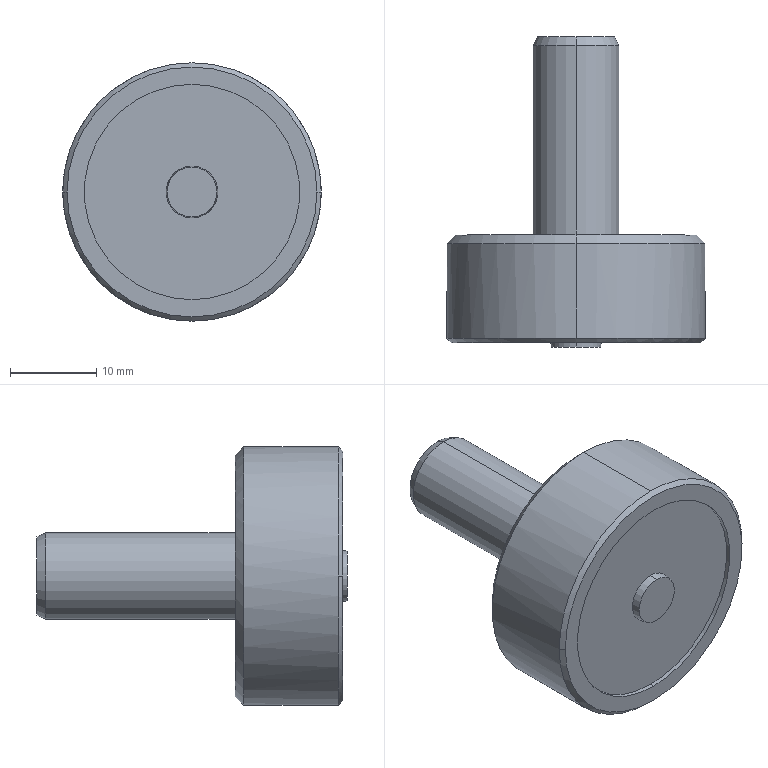Part | SolidWorks | features BaseBody 1 | 1 solid | 19 faces | box 30 x 36 x 30 mm | volume 10359 mm3 | cone 8 | cylinder 6 | plane 5 | commonest cylinder face diameters 10 x2 25 x2 30 x2
STEP:
#1=CARTESIAN_POINT('',(-257.5,37.,118.121));
#2=VERTEX_POINT('',#1);
#3=CARTESIAN_POINT('',(-257.5,37.,128.121));
#4=VERTEX_POINT('',#3);
#5=CARTESIAN_POINT('',(-257.5,37.,123.121));
#6=DIRECTION('',(0.,-1.,0.));
#7=DIRECTION('',(0.,0.,1.));
#8=AXIS2_PLACEMENT_3D('',#5,#6,#7);
#9=CIRCLE('',#8,5.);
#10=EDGE_CURVE('',#2,#4,#9,.T.);
#11=ORIENTED_EDGE('',*,*,#10,.F.);
#12=CARTESIAN_POINT('',(-257.5,59.,118.121));
#13=VERTEX_POINT('',#12);
#14=CARTESIAN_POINT('',(-257.5,60.,118.121));
#15=DIRECTION('',(0.,1.,0.));
#16=VECTOR('',#15,1000.);
#17=LINE('',#14,#16);
#18=EDGE_CURVE('',#2,#13,#17,.T.);
#19=ORIENTED_EDGE('',*,*,#18,.T.);
#20=CARTESIAN_POINT('',(-257.5,59.,128.121));
#21=VERTEX_POINT('',#20);
#22=CARTESIAN_POINT('',(-257.5,59.,123.121));
#23=DIRECTION('',(0.,-1.,0.));
#24=DIRECTION('',(0.,0.,1.));
#25=AXIS2_PLACEMENT_3D('',#22,#23,#24);
#26=CIRCLE('',#25,5.);
#27=EDGE_CURVE('',#13,#21,#26,.T.);
#28=ORIENTED_EDGE('',*,*,#27,.T.);
#29=CARTESIAN_POINT('',(-257.5,60.,128.121));
#30=DIRECTION('',(0.,1.,0.));
#31=VECTOR('',#30,1000.);
#32=LINE('',#29,#31);
#33=EDGE_CURVE('',#4,#21,#32,.T.);
#34=ORIENTED_EDGE('',*,*,#33,.F.);
#35=EDGE_LOOP('',(#11,#19,#28,#34));
#36=FACE_OUTER_BOUND('',#35,.T.);
#37=CARTESIAN_POINT('',(-257.5,60.,123.121));
#38=DIRECTION('',(0.,1.,0.));
#39=DIRECTION('',(0.,0.,1.));
#40=AXIS2_PLACEMENT_3D('',#37,#38,#39);
#41=CYLINDRICAL_SURFACE('',#40,5.);
#42=ADVANCED_FACE('',(#36),#41,.T.);
#43=CARTESIAN_POINT('',(-257.5,37.,137.121));
#44=VERTEX_POINT('',#43);
#45=CARTESIAN_POINT('',(-257.5,37.,109.121));
#46=VERTEX_POINT('',#45);
#47=CARTESIAN_POINT('',(-257.5,37.,123.121));
#48=DIRECTION('',(0.,1.,0.));
#49=DIRECTION('',(0.,0.,-1.));
#50=AXIS2_PLACEMENT_3D('',#47,#48,#49);
#51=CIRCLE('',#50,14.);
#52=EDGE_CURVE('',#44,#46,#51,.T.);
#53=ORIENTED_EDGE('',*,*,#52,.F.);
#54=CARTESIAN_POINT('',(-257.5,36.,138.121));
#55=VERTEX_POINT('',#54);
#56=CARTESIAN_POINT('',(-257.5,36.,138.121));
#57=DIRECTION('',(0.,-0.7071,0.7071));
#58=VECTOR('',#57,1000.);
#59=LINE('',#56,#58);
#60=EDGE_CURVE('',#44,#55,#59,.T.);
#61=ORIENTED_EDGE('',*,*,#60,.T.);
#62=CARTESIAN_POINT('',(-257.5,36.,108.121));
#63=VERTEX_POINT('',#62);
#64=CARTESIAN_POINT('',(-257.5,36.,123.121));
#65=DIRECTION('',(0.,1.,0.));
#66=DIRECTION('',(-0.05078,0.,-0.9987));
#67=AXIS2_PLACEMENT_3D('',#64,#65,#66);
#68=CIRCLE('',#67,15.);
#69=EDGE_CURVE('',#55,#63,#68,.T.);
#70=ORIENTED_EDGE('',*,*,#69,.T.);
#71=CARTESIAN_POINT('',(-257.5,36.,108.121));
#72=DIRECTION('',(0.,-0.7071,-0.7071));
#73=VECTOR('',#72,1000.);
#74=LINE('',#71,#73);
#75=EDGE_CURVE('',#46,#63,#74,.T.);
#76=ORIENTED_EDGE('',*,*,#75,.F.);
#77=EDGE_LOOP('',(#53,#61,#70,#76));
#78=FACE_OUTER_BOUND('',#77,.T.);
#79=CARTESIAN_POINT('',(-257.5,36.,123.121));
#80=DIRECTION('',(0.,-1.,0.));
#81=DIRECTION('',(0.,0.,-1.));
#82=AXIS2_PLACEMENT_3D('',#79,#80,#81);
#83=CONICAL_SURFACE('',#82,15.,0.7854);
#84=ADVANCED_FACE('',(#78),#83,.T.);
#85=CARTESIAN_POINT('',(-257.5,60.,118.587));
#86=VERTEX_POINT('',#85);
#87=CARTESIAN_POINT('',(-257.5,60.,127.655));
#88=VERTEX_POINT('',#87);
#89=CARTESIAN_POINT('',(-257.5,60.,123.121));
#90=DIRECTION('',(0.,-1.,0.));
#91=DIRECTION('',(0.,0.,-1.));
#92=AXIS2_PLACEMENT_3D('',#89,#90,#91);
#93=CIRCLE('',#92,4.534);
#94=EDGE_CURVE('',#86,#88,#93,.T.);
#95=ORIENTED_EDGE('',*,*,#94,.T.);
#96=CARTESIAN_POINT('',(-257.5,59.,128.121));
#97=DIRECTION('',(0.,-0.9063,0.4226));
#98=VECTOR('',#97,1000.);
#99=LINE('',#96,#98);
#100=EDGE_CURVE('',#88,#21,#99,.T.);
#101=ORIENTED_EDGE('',*,*,#100,.T.);
#102=ORIENTED_EDGE('',*,*,#27,.F.);
#103=CARTESIAN_POINT('',(-257.5,59.,118.121));
#104=DIRECTION('',(0.,-0.9063,-0.4226));
#105=VECTOR('',#104,1000.);
#106=LINE('',#103,#105);
#107=EDGE_CURVE('',#86,#13,#106,.T.);
#108=ORIENTED_EDGE('',*,*,#107,.F.);
#109=EDGE_LOOP('',(#95,#101,#102,#108));
#110=FACE_OUTER_BOUND('',#109,.T.);
#111=CARTESIAN_POINT('',(-257.5,59.,123.121));
#112=DIRECTION('',(0.,-1.,0.));
#113=DIRECTION('',(0.,0.,-1.));
#114=AXIS2_PLACEMENT_3D('',#111,#112,#113);
#115=CONICAL_SURFACE('',#114,5.,0.4363);
#116=ADVANCED_FACE('',(#110),#115,.T.);
#117=CARTESIAN_POINT('',(-242.5,25.,123.121));
#118=VERTEX_POINT('',#117);
#119=CARTESIAN_POINT('',(-257.5,25.,108.121));
#120=VERTEX_POINT('',#119);
#121=CARTESIAN_POINT('',(-257.5,25.,123.121));
#122=DIRECTION('',(0.,1.,0.));
#123=DIRECTION('',(0.,0.,1.));
#124=AXIS2_PLACEMENT_3D('',#121,#122,#123);
#125=CIRCLE('',#124,15.);
#126=EDGE_CURVE('',#118,#120,#125,.T.);
#127=ORIENTED_EDGE('',*,*,#126,.T.);
#128=CARTESIAN_POINT('',(-257.5,60.,108.121));
#129=DIRECTION('',(0.,1.,0.));
#130=VECTOR('',#129,1000.);
#131=LINE('',#128,#130);
#132=EDGE_CURVE('',#120,#63,#131,.T.);
#133=ORIENTED_EDGE('',*,*,#132,.T.);
#134=ORIENTED_EDGE('',*,*,#69,.F.);
#135=CARTESIAN_POINT('',(-257.5,25.,138.121));
#136=VERTEX_POINT('',#135);
#137=CARTESIAN_POINT('',(-257.5,60.,138.121));
#138=DIRECTION('',(0.,1.,0.));
#139=VECTOR('',#138,1000.);
#140=LINE('',#137,#139);
#141=EDGE_CURVE('',#136,#55,#140,.T.);
#142=ORIENTED_EDGE('',*,*,#141,.F.);
#143=CARTESIAN_POINT('',(-257.5,25.,123.121));
#144=DIRECTION('',(0.,1.,0.));
#145=DIRECTION('',(0.,0.,1.));
#146=AXIS2_PLACEMENT_3D('',#143,#144,#145);
#147=CIRCLE('',#146,15.);
#148=EDGE_CURVE('',#136,#118,#147,.T.);
#149=ORIENTED_EDGE('',*,*,#148,.T.);
#150=EDGE_LOOP('',(#127,#133,#134,#142,#149));
#151=FACE_OUTER_BOUND('',#150,.T.);
#152=CARTESIAN_POINT('',(-257.5,60.,123.121));
#153=DIRECTION('',(0.,1.,0.));
#154=DIRECTION('',(0.,0.,1.));
#155=AXIS2_PLACEMENT_3D('',#152,#153,#154);
#156=CYLINDRICAL_SURFACE('',#155,15.);
#157=ADVANCED_FACE('',(#151),#156,.T.);
#158=CARTESIAN_POINT('',(-272.,24.5,123.121));
#159=VERTEX_POINT('',#158);
#160=CARTESIAN_POINT('',(-243.,24.5,123.121));
#161=VERTEX_POINT('',#160);
#162=CARTESIAN_POINT('',(-257.5,24.5,123.121));
#163=DIRECTION('',(0.,1.,0.));
#164=DIRECTION('',(-1.,0.,0.));
#165=AXIS2_PLACEMENT_3D('',#162,#163,#164);
#166=CIRCLE('',#165,14.5);
#167=EDGE_CURVE('',#159,#161,#166,.T.);
#168=ORIENTED_EDGE('',*,*,#167,.T.);
#169=CARTESIAN_POINT('',(-242.5,25.,123.121));
#170=DIRECTION('',(0.7071,0.7071,0.));
#171=VECTOR('',#170,1000.);
#172=LINE('',#169,#171);
#173=EDGE_CURVE('',#161,#118,#172,.T.);
#174=ORIENTED_EDGE('',*,*,#173,.T.);
#175=ORIENTED_EDGE('',*,*,#148,.F.);
#176=CARTESIAN_POINT('',(-272.5,25.,123.121));
#177=VERTEX_POINT('',#176);
#178=CARTESIAN_POINT('',(-257.5,25.,123.121));
#179=DIRECTION('',(0.,1.,0.));
#180=DIRECTION('',(0.,0.,1.));
#181=AXIS2_PLACEMENT_3D('',#178,#179,#180);
#182=CIRCLE('',#181,15.);
#183=EDGE_CURVE('',#177,#136,#182,.T.);
#184=ORIENTED_EDGE('',*,*,#183,.F.);
#185=CARTESIAN_POINT('',(-272.5,25.,123.121));
#186=DIRECTION('',(-0.7071,0.7071,0.));
#187=VECTOR('',#186,1000.);
#188=LINE('',#185,#187);
#189=EDGE_CURVE('',#159,#177,#188,.T.);
#190=ORIENTED_EDGE('',*,*,#189,.F.);
#191=EDGE_LOOP('',(#168,#174,#175,#184,#190));
#192=FACE_OUTER_BOUND('',#191,.T.);
#193=CARTESIAN_POINT('',(-257.5,25.,123.121));
#194=DIRECTION('',(0.,1.,0.));
#195=DIRECTION('',(-1.,0.,0.));
#196=AXIS2_PLACEMENT_3D('',#193,#194,#195);
#197=CONICAL_SURFACE('',#196,15.,0.7854);
#198=ADVANCED_FACE('',(#192),#197,.T.);
#199=CARTESIAN_POINT('',(-257.5,25.,135.621));
#200=VERTEX_POINT('',#199);
#201=CARTESIAN_POINT('',(-257.5,25.,110.621));
#202=VERTEX_POINT('',#201);
#203=CARTESIAN_POINT('',(-257.5,25.,123.121));
#204=DIRECTION('',(0.,-1.,0.));
#205=DIRECTION('',(0.,0.,-1.));
#206=AXIS2_PLACEMENT_3D('',#203,#204,#205);
#207=CIRCLE('',#206,12.5);
#208=EDGE_CURVE('',#200,#202,#207,.T.);
#209=ORIENTED_EDGE('',*,*,#208,.F.);
#210=CARTESIAN_POINT('',(-257.5,24.5,135.621));
#211=VERTEX_POINT('',#210);
#212=CARTESIAN_POINT('',(-257.5,25.,135.621));
#213=DIRECTION('',(0.,-1.,0.));
#214=VECTOR('',#213,1000.);
#215=LINE('',#212,#214);
#216=EDGE_CURVE('',#200,#211,#215,.T.);
#217=ORIENTED_EDGE('',*,*,#216,.T.);
#218=CARTESIAN_POINT('',(-257.5,24.5,110.621));
#219=VERTEX_POINT('',#218);
#220=CARTESIAN_POINT('',(-257.5,24.5,123.121));
#221=DIRECTION('',(0.,1.,0.));
#222=DIRECTION('',(0.,0.,-1.));
#223=AXIS2_PLACEMENT_3D('',#220,#221,#222);
#224=CIRCLE('',#223,12.5);
#225=EDGE_CURVE('',#219,#211,#224,.T.);
#226=ORIENTED_EDGE('',*,*,#225,.F.);
#227=CARTESIAN_POINT('',(-257.5,25.,110.621));
#228=DIRECTION('',(0.,-1.,0.));
#229=VECTOR('',#228,1000.);
#230=LINE('',#227,#229);
#231=EDGE_CURVE('',#202,#219,#230,.T.);
#232=ORIENTED_EDGE('',*,*,#231,.F.);
#233=EDGE_LOOP('',(#209,#217,#226,#232));
#234=FACE_OUTER_BOUND('',#233,.T.);
#235=CARTESIAN_POINT('',(-257.5,25.,123.121));
#236=DIRECTION('',(0.,-1.,0.));
#237=DIRECTION('',(0.,0.,-1.));
#238=AXIS2_PLACEMENT_3D('',#235,#236,#237);
#239=CYLINDRICAL_SURFACE('',#238,12.5);
#240=ADVANCED_FACE('',(#234),#239,.F.);
#241=CARTESIAN_POINT('',(-257.5,24.,126.016));
#242=VERTEX_POINT('',#241);
#243=CARTESIAN_POINT('',(-257.5,24.,120.226));
#244=VERTEX_POINT('',#243);
#245=CARTESIAN_POINT('',(-257.5,24.,123.121));
#246=DIRECTION('',(0.,1.,0.));
#247=DIRECTION('',(0.,0.,1.));
#248=AXIS2_PLACEMENT_3D('',#245,#246,#247);
#249=CIRCLE('',#248,2.895);
#250=EDGE_CURVE('',#242,#244,#249,.T.);
#251=ORIENTED_EDGE('',*,*,#250,.T.);
#252=CARTESIAN_POINT('',(-257.5,25.,120.121));
#253=VERTEX_POINT('',#252);
#254=CARTESIAN_POINT('',(-257.5,25.,120.121));
#255=DIRECTION('',(0.,0.9945,-0.1045));
#256=VECTOR('',#255,1000.);
#257=LINE('',#254,#256);
#258=EDGE_CURVE('',#244,#253,#257,.T.);
#259=ORIENTED_EDGE('',*,*,#258,.T.);
#260=CARTESIAN_POINT('',(-257.5,25.,126.121));
#261=VERTEX_POINT('',#260);
#262=CARTESIAN_POINT('',(-257.5,25.,123.121));
#263=DIRECTION('',(0.,1.,0.));
#264=DIRECTION('',(0.,0.,1.));
#265=AXIS2_PLACEMENT_3D('',#262,#263,#264);
#266=CIRCLE('',#265,3.);
#267=EDGE_CURVE('',#261,#253,#266,.T.);
#268=ORIENTED_EDGE('',*,*,#267,.F.);
#269=CARTESIAN_POINT('',(-257.5,25.,126.121));
#270=DIRECTION('',(0.,0.9945,0.1045));
#271=VECTOR('',#270,1000.);
#272=LINE('',#269,#271);
#273=EDGE_CURVE('',#242,#261,#272,.T.);
#274=ORIENTED_EDGE('',*,*,#273,.F.);
#275=EDGE_LOOP('',(#251,#259,#268,#274));
#276=FACE_OUTER_BOUND('',#275,.T.);
#277=CARTESIAN_POINT('',(-257.5,25.,123.121));
#278=DIRECTION('',(0.,1.,0.));
#279=DIRECTION('',(0.,0.,1.));
#280=AXIS2_PLACEMENT_3D('',#277,#278,#279);
#281=CONICAL_SURFACE('',#280,3.,0.1047);
#282=ADVANCED_FACE('',(#276),#281,.T.);
#283=CARTESIAN_POINT('',(-257.5,37.,123.121));
#284=DIRECTION('',(0.,-1.,0.));
#285=DIRECTION('',(0.,0.,1.));
#286=AXIS2_PLACEMENT_3D('',#283,#284,#285);
#287=CIRCLE('',#286,5.);
#288=EDGE_CURVE('',#4,#2,#287,.T.);
#289=ORIENTED_EDGE('',*,*,#288,.T.);
#290=ORIENTED_EDGE('',*,*,#10,.T.);
#291=EDGE_LOOP('',(#289,#290));
#292=FACE_BOUND('',#291,.T.);
#293=CARTESIAN_POINT('',(-257.5,37.,123.121));
#294=DIRECTION('',(0.,1.,0.));
#295=DIRECTION('',(0.,0.,-1.));
#296=AXIS2_PLACEMENT_3D('',#293,#294,#295);
#297=CIRCLE('',#296,14.);
#298=EDGE_CURVE('',#46,#44,#297,.T.);
#299=ORIENTED_EDGE('',*,*,#298,.T.);
#300=ORIENTED_EDGE('',*,*,#52,.T.);
#301=EDGE_LOOP('',(#299,#300));
#302=FACE_OUTER_BOUND('',#301,.T.);
#303=CARTESIAN_POINT('',(-256.738,37.,138.102));
#304=DIRECTION('',(0.,1.,0.));
#305=DIRECTION('',(0.,0.,1.));
#306=AXIS2_PLACEMENT_3D('',#303,#304,#305);
#307=PLANE('',#306);
#308=ADVANCED_FACE('',(#292,#302),#307,.T.);
#309=ORIENTED_EDGE('',*,*,#18,.F.);
#310=ORIENTED_EDGE('',*,*,#288,.F.);
#311=ORIENTED_EDGE('',*,*,#33,.T.);
#312=CARTESIAN_POINT('',(-257.5,59.,123.121));
#313=DIRECTION('',(0.,-1.,0.));
#314=DIRECTION('',(0.,0.,1.));
#315=AXIS2_PLACEMENT_3D('',#312,#313,#314);
#316=CIRCLE('',#315,5.);
#317=EDGE_CURVE('',#21,#13,#316,.T.);
#318=ORIENTED_EDGE('',*,*,#317,.T.);
#319=EDGE_LOOP('',(#309,#310,#311,#318));
#320=FACE_OUTER_BOUND('',#319,.T.);
#321=CARTESIAN_POINT('',(-257.5,60.,123.121));
#322=DIRECTION('',(0.,1.,0.));
#323=DIRECTION('',(0.,0.,1.));
#324=AXIS2_PLACEMENT_3D('',#321,#322,#323);
#325=CYLINDRICAL_SURFACE('',#324,5.);
#326=ADVANCED_FACE('',(#320),#325,.T.);
#327=ORIENTED_EDGE('',*,*,#60,.F.);
#328=ORIENTED_EDGE('',*,*,#298,.F.);
#329=ORIENTED_EDGE('',*,*,#75,.T.);
#330=CARTESIAN_POINT('',(-257.5,36.,123.121));
#331=DIRECTION('',(0.,1.,0.));
#332=DIRECTION('',(-0.05078,0.,-0.9987));
#333=AXIS2_PLACEMENT_3D('',#330,#331,#332);
#334=CIRCLE('',#333,15.);
#335=EDGE_CURVE('',#63,#55,#334,.T.);
#336=ORIENTED_EDGE('',*,*,#335,.T.);
#337=EDGE_LOOP('',(#327,#328,#329,#336));
#338=FACE_OUTER_BOUND('',#337,.T.);
#339=CARTESIAN_POINT('',(-257.5,36.,123.121));
#340=DIRECTION('',(0.,-1.,0.));
#341=DIRECTION('',(0.,0.,-1.));
#342=AXIS2_PLACEMENT_3D('',#339,#340,#341);
#343=CONICAL_SURFACE('',#342,15.,0.7854);
#344=ADVANCED_FACE('',(#338),#343,.T.);
#345=ORIENTED_EDGE('',*,*,#100,.F.);
#346=CARTESIAN_POINT('',(-257.5,60.,123.121));
#347=DIRECTION('',(0.,-1.,0.));
#348=DIRECTION('',(0.,0.,-1.));
#349=AXIS2_PLACEMENT_3D('',#346,#347,#348);
#350=CIRCLE('',#349,4.534);
#351=EDGE_CURVE('',#88,#86,#350,.T.);
#352=ORIENTED_EDGE('',*,*,#351,.T.);
#353=ORIENTED_EDGE('',*,*,#107,.T.);
#354=ORIENTED_EDGE('',*,*,#317,.F.);
#355=EDGE_LOOP('',(#345,#352,#353,#354));
#356=FACE_OUTER_BOUND('',#355,.T.);
#357=CARTESIAN_POINT('',(-257.5,59.,123.121));
#358=DIRECTION('',(0.,-1.,0.));
#359=DIRECTION('',(0.,0.,-1.));
#360=AXIS2_PLACEMENT_3D('',#357,#358,#359);
#361=CONICAL_SURFACE('',#360,5.,0.4363);
#362=ADVANCED_FACE('',(#356),#361,.T.);
#363=ORIENTED_EDGE('',*,*,#132,.F.);
#364=CARTESIAN_POINT('',(-257.5,25.,123.121));
#365=DIRECTION('',(0.,1.,0.));
#366=DIRECTION('',(0.,0.,1.));
#367=AXIS2_PLACEMENT_3D('',#364,#365,#366);
#368=CIRCLE('',#367,15.);
#369=EDGE_CURVE('',#120,#177,#368,.T.);
#370=ORIENTED_EDGE('',*,*,#369,.T.);
#371=ORIENTED_EDGE('',*,*,#183,.T.);
#372=ORIENTED_EDGE('',*,*,#141,.T.);
#373=ORIENTED_EDGE('',*,*,#335,.F.);
#374=EDGE_LOOP('',(#363,#370,#371,#372,#373));
#375=FACE_OUTER_BOUND('',#374,.T.);
#376=CARTESIAN_POINT('',(-257.5,60.,123.121));
#377=DIRECTION('',(0.,1.,0.));
#378=DIRECTION('',(0.,0.,1.));
#379=AXIS2_PLACEMENT_3D('',#376,#377,#378);
#380=CYLINDRICAL_SURFACE('',#379,15.);
#381=ADVANCED_FACE('',(#375),#380,.T.);
#382=ORIENTED_EDGE('',*,*,#94,.F.);
#383=ORIENTED_EDGE('',*,*,#351,.F.);
#384=EDGE_LOOP('',(#382,#383));
#385=FACE_OUTER_BOUND('',#384,.T.);
#386=CARTESIAN_POINT('',(-257.246,60.,128.115));
#387=DIRECTION('',(0.,1.,0.));
#388=DIRECTION('',(0.,0.,1.));
#389=AXIS2_PLACEMENT_3D('',#386,#387,#388);
#390=PLANE('',#389);
#391=ADVANCED_FACE('',(#385),#390,.T.);
#392=ORIENTED_EDGE('',*,*,#173,.F.);
#393=CARTESIAN_POINT('',(-257.5,24.5,123.121));
#394=DIRECTION('',(0.,1.,0.));
#395=DIRECTION('',(-1.,0.,0.));
#396=AXIS2_PLACEMENT_3D('',#393,#394,#395);
#397=CIRCLE('',#396,14.5);
#398=EDGE_CURVE('',#161,#159,#397,.T.);
#399=ORIENTED_EDGE('',*,*,#398,.T.);
#400=ORIENTED_EDGE('',*,*,#189,.T.);
#401=ORIENTED_EDGE('',*,*,#369,.F.);
#402=ORIENTED_EDGE('',*,*,#126,.F.);
#403=EDGE_LOOP('',(#392,#399,#400,#401,#402));
#404=FACE_OUTER_BOUND('',#403,.T.);
#405=CARTESIAN_POINT('',(-257.5,25.,123.121));
#406=DIRECTION('',(0.,1.,0.));
#407=DIRECTION('',(-1.,0.,0.));
#408=AXIS2_PLACEMENT_3D('',#405,#406,#407);
#409=CONICAL_SURFACE('',#408,15.,0.7854);
#410=ADVANCED_FACE('',(#404),#409,.T.);
#411=ORIENTED_EDGE('',*,*,#167,.F.);
#412=ORIENTED_EDGE('',*,*,#398,.F.);
#413=EDGE_LOOP('',(#411,#412));
#414=FACE_OUTER_BOUND('',#413,.T.);
#415=ORIENTED_EDGE('',*,*,#225,.T.);
#416=CARTESIAN_POINT('',(-257.5,24.5,123.121));
#417=DIRECTION('',(0.,1.,0.));
#418=DIRECTION('',(0.,0.,-1.));
#419=AXIS2_PLACEMENT_3D('',#416,#417,#418);
#420=CIRCLE('',#419,12.5);
#421=EDGE_CURVE('',#211,#219,#420,.T.);
#422=ORIENTED_EDGE('',*,*,#421,.T.);
#423=EDGE_LOOP('',(#415,#422));
#424=FACE_BOUND('',#423,.T.);
#425=CARTESIAN_POINT('',(-257.5,24.5,123.121));
#426=DIRECTION('',(0.,-1.,0.));
#427=DIRECTION('',(0.,0.,-1.));
#428=AXIS2_PLACEMENT_3D('',#425,#426,#427);
#429=PLANE('',#428);
#430=ADVANCED_FACE('',(#414,#424),#429,.T.);
#431=ORIENTED_EDGE('',*,*,#216,.F.);
#432=CARTESIAN_POINT('',(-257.5,25.,123.121));
#433=DIRECTION('',(0.,-1.,0.));
#434=DIRECTION('',(0.,0.,-1.));
#435=AXIS2_PLACEMENT_3D('',#432,#433,#434);
#436=CIRCLE('',#435,12.5);
#437=EDGE_CURVE('',#202,#200,#436,.T.);
#438=ORIENTED_EDGE('',*,*,#437,.F.);
#439=ORIENTED_EDGE('',*,*,#231,.T.);
#440=ORIENTED_EDGE('',*,*,#421,.F.);
#441=EDGE_LOOP('',(#431,#438,#439,#440));
#442=FACE_OUTER_BOUND('',#441,.T.);
#443=CARTESIAN_POINT('',(-257.5,25.,123.121));
#444=DIRECTION('',(0.,-1.,0.));
#445=DIRECTION('',(0.,0.,-1.));
#446=AXIS2_PLACEMENT_3D('',#443,#444,#445);
#447=CYLINDRICAL_SURFACE('',#446,12.5);
#448=ADVANCED_FACE('',(#442),#447,.F.);
#449=ORIENTED_EDGE('',*,*,#267,.T.);
#450=CARTESIAN_POINT('',(-257.5,25.,123.121));
#451=DIRECTION('',(0.,1.,0.));
#452=DIRECTION('',(0.,0.,1.));
#453=AXIS2_PLACEMENT_3D('',#450,#451,#452);
#454=CIRCLE('',#453,3.);
#455=EDGE_CURVE('',#253,#261,#454,.T.);
#456=ORIENTED_EDGE('',*,*,#455,.T.);
#457=EDGE_LOOP('',(#449,#456));
#458=FACE_BOUND('',#457,.T.);
#459=ORIENTED_EDGE('',*,*,#437,.T.);
#460=ORIENTED_EDGE('',*,*,#208,.T.);
#461=EDGE_LOOP('',(#459,#460));
#462=FACE_OUTER_BOUND('',#461,.T.);
#463=CARTESIAN_POINT('',(-257.5,25.,123.121));
#464=DIRECTION('',(0.,-1.,0.));
#465=DIRECTION('',(0.,0.,-1.));
#466=AXIS2_PLACEMENT_3D('',#463,#464,#465);
#467=PLANE('',#466);
#468=ADVANCED_FACE('',(#458,#462),#467,.T.);
#469=ORIENTED_EDGE('',*,*,#258,.F.);
#470=CARTESIAN_POINT('',(-257.5,24.,123.121));
#471=DIRECTION('',(0.,1.,0.));
#472=DIRECTION('',(0.,0.,1.));
#473=AXIS2_PLACEMENT_3D('',#470,#471,#472);
#474=CIRCLE('',#473,2.895);
#475=EDGE_CURVE('',#244,#242,#474,.T.);
#476=ORIENTED_EDGE('',*,*,#475,.T.);
#477=ORIENTED_EDGE('',*,*,#273,.T.);
#478=ORIENTED_EDGE('',*,*,#455,.F.);
#479=EDGE_LOOP('',(#469,#476,#477,#478));
#480=FACE_OUTER_BOUND('',#479,.T.);
#481=CARTESIAN_POINT('',(-257.5,25.,123.121));
#482=DIRECTION('',(0.,1.,0.));
#483=DIRECTION('',(0.,0.,1.));
#484=AXIS2_PLACEMENT_3D('',#481,#482,#483);
#485=CONICAL_SURFACE('',#484,3.,0.1047);
#486=ADVANCED_FACE('',(#480),#485,.T.);
#487=ORIENTED_EDGE('',*,*,#250,.F.);
#488=ORIENTED_EDGE('',*,*,#475,.F.);
#489=EDGE_LOOP('',(#487,#488));
#490=FACE_OUTER_BOUND('',#489,.T.);
#491=CARTESIAN_POINT('',(-257.5,24.,123.121));
#492=DIRECTION('',(0.,-1.,0.));
#493=DIRECTION('',(0.,0.,-1.));
#494=AXIS2_PLACEMENT_3D('',#491,#492,#493);
#495=PLANE('',#494);
#496=ADVANCED_FACE('',(#490),#495,.T.);
#497=CLOSED_SHELL('',(#42,#84,#116,#157,#198,#240,#282,#308,#326,#344,#362,#381,#391,#410,#430,#448,#468,#486,#496));
#498=MANIFOLD_SOLID_BREP('',#497);
#499=CARTESIAN_POINT('',(0.,0.,0.));
#500=DIRECTION('',(0.,0.,1.));
#501=DIRECTION('',(1.,0.,0.));
#502=AXIS2_PLACEMENT_3D('',#499,#500,#501);
#503=(LENGTH_UNIT()NAMED_UNIT(*)SI_UNIT(.MILLI.,.METRE.));
#504=UNCERTAINTY_MEASURE_WITH_UNIT(LENGTH_MEASURE(0.00001),#503,'','');
#505=(NAMED_UNIT(*)PLANE_ANGLE_UNIT()SI_UNIT($,.RADIAN.));
#506=(NAMED_UNIT(*)SI_UNIT($,.STERADIAN.)SOLID_ANGLE_UNIT());
#507=(GEOMETRIC_REPRESENTATION_CONTEXT(3)GLOBAL_UNCERTAINTY_ASSIGNED_CONTEXT((#504))GLOBAL_UNIT_ASSIGNED_CONTEXT((#503,#505,#506))REPRESENTATION_CONTEXT('',''));
#508=ADVANCED_BREP_SHAPE_REPRESENTATION('',(#498,#502),#507);